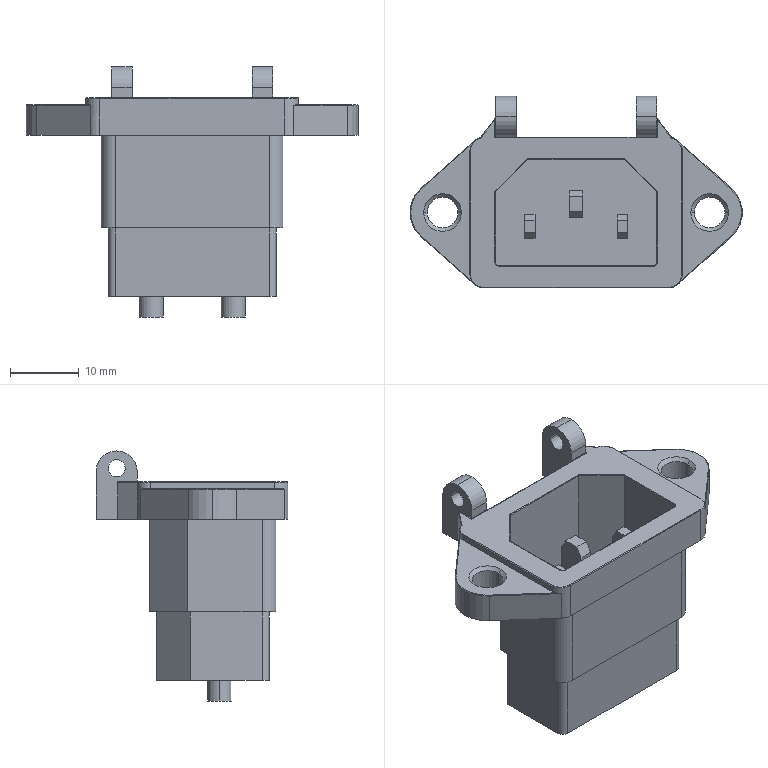Part | SolidWorks | features BaseBody 1 | 1 solid | 130 faces | box 48.5 x 28 x 36.5 mm | volume 8640 mm3 | plane 66 | cylinder 49 | torus 9 | cone 4 | spline 2 | commonest cylinder face diameters 0.2 x20 4 x6 2.5 x4 3.5 x4 4.5 x4 6 x4